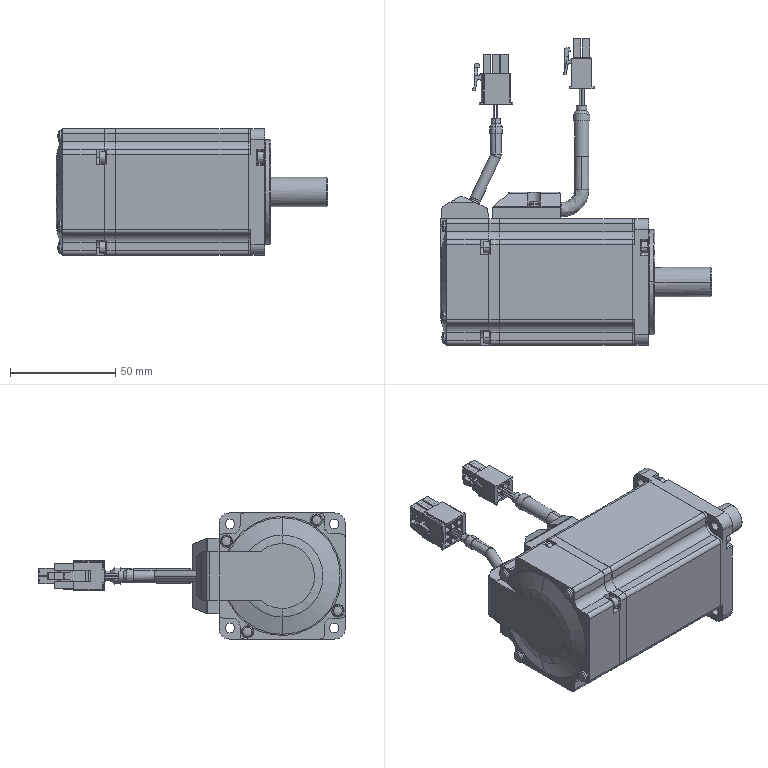Part | SolidWorks | 7 solids | 948 faces | box 129 x 145.682 x 60 mm | volume 347551 mm3 | plane 552 | cylinder 299 | cone 59 | spline 34 | torus 4 | commonest cylinder face diameters 1 x35 4 x33 6 x29 2.6 x26 3.92 x20 5.5 x16